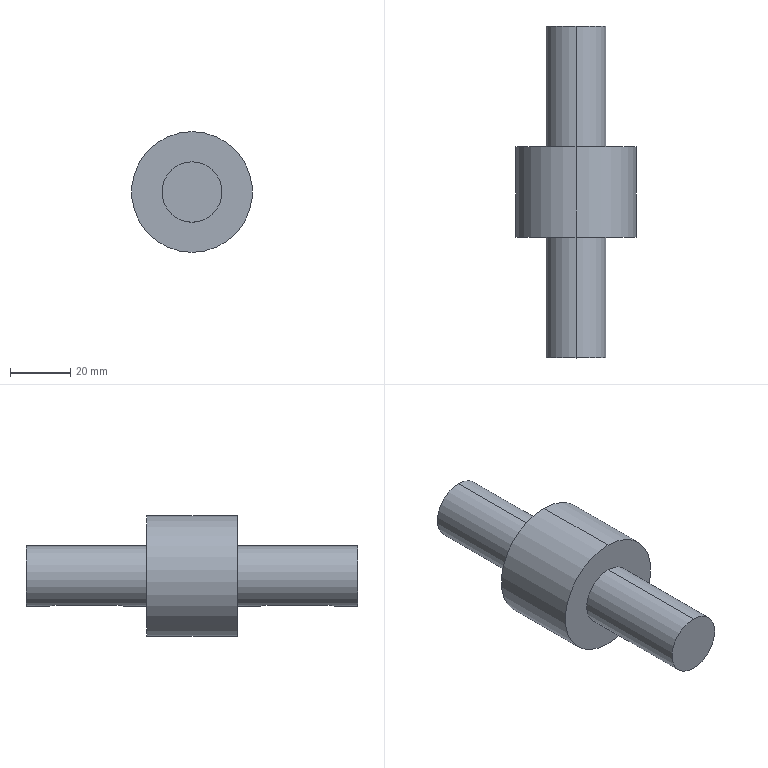Part | SolidWorks | features ICE 1, MirrorPattern 1, Revolution 1 | 1 solid | 20 faces | box 40 x 110 x 40 mm | volume 62258 mm3 | cylinder 10 | plane 10 | commonest cylinder face diameters 5 x4 20 x4 40 x2
STEP:
#1=CARTESIAN_POINT('',(0.,-15.,20.));
#2=VERTEX_POINT('',#1);
#3=CARTESIAN_POINT('',(0.,-15.,-20.));
#4=VERTEX_POINT('',#3);
#5=CARTESIAN_POINT('',(0.,-15.,0.));
#6=DIRECTION('',(0.,1.,0.));
#7=DIRECTION('',(0.,0.,1.));
#8=AXIS2_PLACEMENT_3D('',#5,#6,#7);
#9=CIRCLE('',#8,20.);
#10=EDGE_CURVE('',#2,#4,#9,.T.);
#11=ORIENTED_EDGE('',*,*,#10,.T.);
#12=CARTESIAN_POINT('',(0.,15.,-20.));
#13=VERTEX_POINT('',#12);
#14=CARTESIAN_POINT('',(0.,189.93,-20.));
#15=DIRECTION('',(0.,1.,0.));
#16=VECTOR('',#15,1000.);
#17=LINE('',#14,#16);
#18=EDGE_CURVE('',#4,#13,#17,.T.);
#19=ORIENTED_EDGE('',*,*,#18,.T.);
#20=CARTESIAN_POINT('',(0.,15.,20.));
#21=VERTEX_POINT('',#20);
#22=CARTESIAN_POINT('',(0.,15.,0.));
#23=DIRECTION('',(0.,1.,0.));
#24=DIRECTION('',(0.,0.,1.));
#25=AXIS2_PLACEMENT_3D('',#22,#23,#24);
#26=CIRCLE('',#25,20.);
#27=EDGE_CURVE('',#21,#13,#26,.T.);
#28=ORIENTED_EDGE('',*,*,#27,.F.);
#29=CARTESIAN_POINT('',(0.,189.93,20.));
#30=DIRECTION('',(0.,1.,0.));
#31=VECTOR('',#30,1000.);
#32=LINE('',#29,#31);
#33=EDGE_CURVE('',#2,#21,#32,.T.);
#34=ORIENTED_EDGE('',*,*,#33,.F.);
#35=EDGE_LOOP('',(#11,#19,#28,#34));
#36=FACE_OUTER_BOUND('',#35,.T.);
#37=CARTESIAN_POINT('',(0.,189.93,0.));
#38=DIRECTION('',(0.,1.,0.));
#39=DIRECTION('',(0.,0.,1.));
#40=AXIS2_PLACEMENT_3D('',#37,#38,#39);
#41=CYLINDRICAL_SURFACE('',#40,20.);
#42=ADVANCED_FACE('',(#36),#41,.T.);
#43=CARTESIAN_POINT('',(0.,15.,10.));
#44=VERTEX_POINT('',#43);
#45=CARTESIAN_POINT('',(0.,15.,-10.));
#46=VERTEX_POINT('',#45);
#47=CARTESIAN_POINT('',(0.,15.,0.));
#48=DIRECTION('',(0.,1.,0.));
#49=DIRECTION('',(0.,0.,1.));
#50=AXIS2_PLACEMENT_3D('',#47,#48,#49);
#51=CIRCLE('',#50,10.);
#52=EDGE_CURVE('',#44,#46,#51,.T.);
#53=ORIENTED_EDGE('',*,*,#52,.T.);
#54=CARTESIAN_POINT('',(0.,22.5,-10.));
#55=VERTEX_POINT('',#54);
#56=CARTESIAN_POINT('',(0.,189.93,-10.));
#57=DIRECTION('',(0.,1.,0.));
#58=VECTOR('',#57,1000.);
#59=LINE('',#56,#58);
#60=EDGE_CURVE('',#46,#55,#59,.T.);
#61=ORIENTED_EDGE('',*,*,#60,.T.);
#62=CARTESIAN_POINT('',(2.5,25.,-9.682));
#63=VERTEX_POINT('',#62);
#64=CARTESIAN_POINT('',(2.5,25.,-9.682));
#65=CARTESIAN_POINT('',(2.5,24.834,-9.682));
#66=CARTESIAN_POINT('',(2.484,24.671,-9.687));
#67=CARTESIAN_POINT('',(2.42,24.351,-9.703));
#68=CARTESIAN_POINT('',(2.371,24.191,-9.715));
#69=CARTESIAN_POINT('',(2.245,23.889,-9.745));
#70=CARTESIAN_POINT('',(2.169,23.745,-9.762));
#71=CARTESIAN_POINT('',(1.987,23.474,-9.801));
#72=CARTESIAN_POINT('',(1.882,23.346,-9.822));
#73=CARTESIAN_POINT('',(1.537,23.002,-9.884));
#74=CARTESIAN_POINT('',(1.259,22.816,-9.925));
#75=CARTESIAN_POINT('',(0.8081,22.629,-9.968));
#76=CARTESIAN_POINT('',(0.6497,22.58,-9.98));
#77=CARTESIAN_POINT('',(0.3266,22.516,-9.996));
#78=CARTESIAN_POINT('',(0.1638,22.5,-10.));
#79=CARTESIAN_POINT('',(0.,22.5,-10.));
#80=B_SPLINE_CURVE_WITH_KNOTS('',3,(#64,#65,#66,#67,#68,#69,#70,#71,#72,#73,#74,#75,#76,#77,#78,#79),.UNSPECIFIED.,.F.,.F.,(4,2,2,2,2,2,2,4),(0.,0.0004906,0.0009812,0.001472,0.001962,0.002944,0.003434,0.003925),.UNSPECIFIED.);
#81=EDGE_CURVE('',#63,#55,#80,.T.);
#82=ORIENTED_EDGE('',*,*,#81,.F.);
#83=CARTESIAN_POINT('',(2.5,45.,-9.682));
#84=VERTEX_POINT('',#83);
#85=CARTESIAN_POINT('',(2.5,189.93,-9.682));
#86=DIRECTION('',(0.,-1.,0.));
#87=VECTOR('',#86,1000.);
#88=LINE('',#85,#87);
#89=EDGE_CURVE('',#84,#63,#88,.T.);
#90=ORIENTED_EDGE('',*,*,#89,.F.);
#91=CARTESIAN_POINT('',(0.,47.5,-10.));
#92=VERTEX_POINT('',#91);
#93=CARTESIAN_POINT('',(0.,47.5,-10.));
#94=CARTESIAN_POINT('',(0.1637,47.5,-10.));
#95=CARTESIAN_POINT('',(0.3299,47.484,-9.996));
#96=CARTESIAN_POINT('',(0.6508,47.419,-9.98));
#97=CARTESIAN_POINT('',(0.8069,47.372,-9.969));
#98=CARTESIAN_POINT('',(1.262,47.183,-9.925));
#99=CARTESIAN_POINT('',(1.536,46.999,-9.884));
#100=CARTESIAN_POINT('',(1.884,46.652,-9.822));
#101=CARTESIAN_POINT('',(1.986,46.527,-9.801));
#102=CARTESIAN_POINT('',(2.167,46.257,-9.763));
#103=CARTESIAN_POINT('',(2.246,46.11,-9.745));
#104=CARTESIAN_POINT('',(2.371,45.809,-9.715));
#105=CARTESIAN_POINT('',(2.419,45.653,-9.703));
#106=CARTESIAN_POINT('',(2.483,45.332,-9.687));
#107=CARTESIAN_POINT('',(2.5,45.166,-9.682));
#108=CARTESIAN_POINT('',(2.5,45.,-9.682));
#109=B_SPLINE_CURVE_WITH_KNOTS('',3,(#93,#94,#95,#96,#97,#98,#99,#100,#101,#102,#103,#104,#105,#106,#107,#108),.UNSPECIFIED.,.F.,.F.,(4,2,2,2,2,2,2,4),(0.003925,0.004415,0.004905,0.005885,0.006375,0.006865,0.007355,0.007845),.UNSPECIFIED.);
#110=EDGE_CURVE('',#92,#84,#109,.T.);
#111=ORIENTED_EDGE('',*,*,#110,.F.);
#112=CARTESIAN_POINT('',(0.,55.,-10.));
#113=VERTEX_POINT('',#112);
#114=CARTESIAN_POINT('',(0.,189.93,-10.));
#115=DIRECTION('',(0.,1.,0.));
#116=VECTOR('',#115,1000.);
#117=LINE('',#114,#116);
#118=EDGE_CURVE('',#92,#113,#117,.T.);
#119=ORIENTED_EDGE('',*,*,#118,.T.);
#120=CARTESIAN_POINT('',(0.,55.,10.));
#121=VERTEX_POINT('',#120);
#122=CARTESIAN_POINT('',(0.,55.,0.));
#123=DIRECTION('',(0.,1.,0.));
#124=DIRECTION('',(0.,0.,1.));
#125=AXIS2_PLACEMENT_3D('',#122,#123,#124);
#126=CIRCLE('',#125,10.);
#127=EDGE_CURVE('',#121,#113,#126,.T.);
#128=ORIENTED_EDGE('',*,*,#127,.F.);
#129=CARTESIAN_POINT('',(0.,189.93,10.));
#130=DIRECTION('',(0.,1.,0.));
#131=VECTOR('',#130,1000.);
#132=LINE('',#129,#131);
#133=EDGE_CURVE('',#44,#121,#132,.T.);
#134=ORIENTED_EDGE('',*,*,#133,.F.);
#135=EDGE_LOOP('',(#53,#61,#82,#90,#111,#119,#128,#134));
#136=FACE_OUTER_BOUND('',#135,.T.);
#137=CARTESIAN_POINT('',(0.,189.93,0.));
#138=DIRECTION('',(0.,1.,0.));
#139=DIRECTION('',(0.,0.,1.));
#140=AXIS2_PLACEMENT_3D('',#137,#138,#139);
#141=CYLINDRICAL_SURFACE('',#140,10.);
#142=ADVANCED_FACE('',(#136),#141,.T.);
#143=CARTESIAN_POINT('',(0.,-55.,10.));
#144=VERTEX_POINT('',#143);
#145=CARTESIAN_POINT('',(0.,-55.,-10.));
#146=VERTEX_POINT('',#145);
#147=CARTESIAN_POINT('',(0.,-55.,0.));
#148=DIRECTION('',(0.,1.,0.));
#149=DIRECTION('',(0.,0.,1.));
#150=AXIS2_PLACEMENT_3D('',#147,#148,#149);
#151=CIRCLE('',#150,10.);
#152=EDGE_CURVE('',#144,#146,#151,.T.);
#153=ORIENTED_EDGE('',*,*,#152,.T.);
#154=CARTESIAN_POINT('',(0.,-47.5,-10.));
#155=VERTEX_POINT('',#154);
#156=CARTESIAN_POINT('',(0.,189.93,-10.));
#157=DIRECTION('',(0.,1.,0.));
#158=VECTOR('',#157,1000.);
#159=LINE('',#156,#158);
#160=EDGE_CURVE('',#146,#155,#159,.T.);
#161=ORIENTED_EDGE('',*,*,#160,.T.);
#162=CARTESIAN_POINT('',(2.5,-45.,-9.682));
#163=VERTEX_POINT('',#162);
#164=CARTESIAN_POINT('',(0.,-47.5,-10.));
#165=CARTESIAN_POINT('',(0.1637,-47.5,-10.));
#166=CARTESIAN_POINT('',(0.3299,-47.484,-9.996));
#167=CARTESIAN_POINT('',(0.6508,-47.419,-9.98));
#168=CARTESIAN_POINT('',(0.8069,-47.372,-9.969));
#169=CARTESIAN_POINT('',(1.262,-47.183,-9.925));
#170=CARTESIAN_POINT('',(1.536,-46.999,-9.884));
#171=CARTESIAN_POINT('',(1.884,-46.652,-9.822));
#172=CARTESIAN_POINT('',(1.986,-46.527,-9.801));
#173=CARTESIAN_POINT('',(2.167,-46.257,-9.763));
#174=CARTESIAN_POINT('',(2.246,-46.11,-9.745));
#175=CARTESIAN_POINT('',(2.371,-45.809,-9.715));
#176=CARTESIAN_POINT('',(2.419,-45.653,-9.703));
#177=CARTESIAN_POINT('',(2.483,-45.332,-9.687));
#178=CARTESIAN_POINT('',(2.5,-45.166,-9.682));
#179=CARTESIAN_POINT('',(2.5,-45.,-9.682));
#180=B_SPLINE_CURVE_WITH_KNOTS('',3,(#164,#165,#166,#167,#168,#169,#170,#171,#172,#173,#174,#175,#176,#177,#178,#179),.UNSPECIFIED.,.F.,.F.,(4,2,2,2,2,2,2,4),(0.003925,0.004415,0.004905,0.005885,0.006375,0.006865,0.007355,0.007845),.UNSPECIFIED.);
#181=EDGE_CURVE('',#155,#163,#180,.T.);
#182=ORIENTED_EDGE('',*,*,#181,.T.);
#183=CARTESIAN_POINT('',(2.5,-25.,-9.682));
#184=VERTEX_POINT('',#183);
#185=CARTESIAN_POINT('',(2.5,189.93,-9.682));
#186=DIRECTION('',(0.,1.,0.));
#187=VECTOR('',#186,1000.);
#188=LINE('',#185,#187);
#189=EDGE_CURVE('',#163,#184,#188,.T.);
#190=ORIENTED_EDGE('',*,*,#189,.T.);
#191=CARTESIAN_POINT('',(0.,-22.5,-10.));
#192=VERTEX_POINT('',#191);
#193=CARTESIAN_POINT('',(2.5,-25.,-9.682));
#194=CARTESIAN_POINT('',(2.5,-24.834,-9.682));
#195=CARTESIAN_POINT('',(2.484,-24.671,-9.687));
#196=CARTESIAN_POINT('',(2.42,-24.351,-9.703));
#197=CARTESIAN_POINT('',(2.371,-24.191,-9.715));
#198=CARTESIAN_POINT('',(2.245,-23.889,-9.745));
#199=CARTESIAN_POINT('',(2.169,-23.745,-9.762));
#200=CARTESIAN_POINT('',(1.987,-23.474,-9.801));
#201=CARTESIAN_POINT('',(1.882,-23.346,-9.822));
#202=CARTESIAN_POINT('',(1.537,-23.002,-9.884));
#203=CARTESIAN_POINT('',(1.259,-22.816,-9.925));
#204=CARTESIAN_POINT('',(0.8081,-22.629,-9.968));
#205=CARTESIAN_POINT('',(0.6497,-22.58,-9.98));
#206=CARTESIAN_POINT('',(0.3266,-22.516,-9.996));
#207=CARTESIAN_POINT('',(0.1638,-22.5,-10.));
#208=CARTESIAN_POINT('',(0.,-22.5,-10.));
#209=B_SPLINE_CURVE_WITH_KNOTS('',3,(#193,#194,#195,#196,#197,#198,#199,#200,#201,#202,#203,#204,#205,#206,#207,#208),.UNSPECIFIED.,.F.,.F.,(4,2,2,2,2,2,2,4),(0.,0.0004906,0.0009812,0.001472,0.001962,0.002944,0.003434,0.003925),.UNSPECIFIED.);
#210=EDGE_CURVE('',#184,#192,#209,.T.);
#211=ORIENTED_EDGE('',*,*,#210,.T.);
#212=CARTESIAN_POINT('',(0.,-15.,-10.));
#213=VERTEX_POINT('',#212);
#214=CARTESIAN_POINT('',(0.,189.93,-10.));
#215=DIRECTION('',(0.,1.,0.));
#216=VECTOR('',#215,1000.);
#217=LINE('',#214,#216);
#218=EDGE_CURVE('',#192,#213,#217,.T.);
#219=ORIENTED_EDGE('',*,*,#218,.T.);
#220=CARTESIAN_POINT('',(0.,-15.,10.));
#221=VERTEX_POINT('',#220);
#222=CARTESIAN_POINT('',(0.,-15.,0.));
#223=DIRECTION('',(0.,1.,0.));
#224=DIRECTION('',(0.,0.,1.));
#225=AXIS2_PLACEMENT_3D('',#222,#223,#224);
#226=CIRCLE('',#225,10.);
#227=EDGE_CURVE('',#221,#213,#226,.T.);
#228=ORIENTED_EDGE('',*,*,#227,.F.);
#229=CARTESIAN_POINT('',(0.,189.93,10.));
#230=DIRECTION('',(0.,1.,0.));
#231=VECTOR('',#230,1000.);
#232=LINE('',#229,#231);
#233=EDGE_CURVE('',#144,#221,#232,.T.);
#234=ORIENTED_EDGE('',*,*,#233,.F.);
#235=EDGE_LOOP('',(#153,#161,#182,#190,#211,#219,#228,#234));
#236=FACE_OUTER_BOUND('',#235,.T.);
#237=CARTESIAN_POINT('',(0.,189.93,0.));
#238=DIRECTION('',(0.,1.,0.));
#239=DIRECTION('',(0.,0.,1.));
#240=AXIS2_PLACEMENT_3D('',#237,#238,#239);
#241=CYLINDRICAL_SURFACE('',#240,10.);
#242=ADVANCED_FACE('',(#236),#241,.T.);
#243=ORIENTED_EDGE('',*,*,#160,.F.);
#244=CARTESIAN_POINT('',(0.,-55.,0.));
#245=DIRECTION('',(0.,1.,0.));
#246=DIRECTION('',(0.,0.,1.));
#247=AXIS2_PLACEMENT_3D('',#244,#245,#246);
#248=CIRCLE('',#247,10.);
#249=EDGE_CURVE('',#146,#144,#248,.T.);
#250=ORIENTED_EDGE('',*,*,#249,.T.);
#251=ORIENTED_EDGE('',*,*,#233,.T.);
#252=CARTESIAN_POINT('',(0.,-15.,0.));
#253=DIRECTION('',(0.,1.,0.));
#254=DIRECTION('',(0.,0.,1.));
#255=AXIS2_PLACEMENT_3D('',#252,#253,#254);
#256=CIRCLE('',#255,10.);
#257=EDGE_CURVE('',#213,#221,#256,.T.);
#258=ORIENTED_EDGE('',*,*,#257,.F.);
#259=ORIENTED_EDGE('',*,*,#218,.F.);
#260=CARTESIAN_POINT('',(-2.5,-25.,-9.682));
#261=VERTEX_POINT('',#260);
#262=CARTESIAN_POINT('',(0.,-22.5,-10.));
#263=CARTESIAN_POINT('',(-0.1637,-22.5,-10.));
#264=CARTESIAN_POINT('',(-0.3299,-22.516,-9.996));
#265=CARTESIAN_POINT('',(-0.6508,-22.581,-9.98));
#266=CARTESIAN_POINT('',(-0.8069,-22.628,-9.969));
#267=CARTESIAN_POINT('',(-1.262,-22.817,-9.925));
#268=CARTESIAN_POINT('',(-1.536,-23.001,-9.884));
#269=CARTESIAN_POINT('',(-1.884,-23.348,-9.822));
#270=CARTESIAN_POINT('',(-1.986,-23.473,-9.801));
#271=CARTESIAN_POINT('',(-2.167,-23.743,-9.763));
#272=CARTESIAN_POINT('',(-2.246,-23.89,-9.745));
#273=CARTESIAN_POINT('',(-2.371,-24.191,-9.715));
#274=CARTESIAN_POINT('',(-2.419,-24.347,-9.703));
#275=CARTESIAN_POINT('',(-2.483,-24.668,-9.687));
#276=CARTESIAN_POINT('',(-2.5,-24.834,-9.682));
#277=CARTESIAN_POINT('',(-2.5,-25.,-9.682));
#278=B_SPLINE_CURVE_WITH_KNOTS('',3,(#262,#263,#264,#265,#266,#267,#268,#269,#270,#271,#272,#273,#274,#275,#276,#277),.UNSPECIFIED.,.F.,.F.,(4,2,2,2,2,2,2,4),(0.003925,0.004415,0.004905,0.005885,0.006375,0.006865,0.007355,0.007845),.UNSPECIFIED.);
#279=EDGE_CURVE('',#192,#261,#278,.T.);
#280=ORIENTED_EDGE('',*,*,#279,.T.);
#281=CARTESIAN_POINT('',(-2.5,-45.,-9.682));
#282=VERTEX_POINT('',#281);
#283=CARTESIAN_POINT('',(-2.5,189.93,-9.682));
#284=DIRECTION('',(0.,-1.,0.));
#285=VECTOR('',#284,1000.);
#286=LINE('',#283,#285);
#287=EDGE_CURVE('',#261,#282,#286,.T.);
#288=ORIENTED_EDGE('',*,*,#287,.T.);
#289=CARTESIAN_POINT('',(-2.5,-45.,-9.682));
#290=CARTESIAN_POINT('',(-2.5,-45.166,-9.682));
#291=CARTESIAN_POINT('',(-2.484,-45.329,-9.687));
#292=CARTESIAN_POINT('',(-2.42,-45.649,-9.703));
#293=CARTESIAN_POINT('',(-2.371,-45.809,-9.715));
#294=CARTESIAN_POINT('',(-2.245,-46.111,-9.745));
#295=CARTESIAN_POINT('',(-2.169,-46.255,-9.762));
#296=CARTESIAN_POINT('',(-1.987,-46.526,-9.801));
#297=CARTESIAN_POINT('',(-1.882,-46.654,-9.822));
#298=CARTESIAN_POINT('',(-1.537,-46.998,-9.884));
#299=CARTESIAN_POINT('',(-1.259,-47.184,-9.925));
#300=CARTESIAN_POINT('',(-0.8081,-47.371,-9.968));
#301=CARTESIAN_POINT('',(-0.6497,-47.42,-9.98));
#302=CARTESIAN_POINT('',(-0.3266,-47.484,-9.996));
#303=CARTESIAN_POINT('',(-0.1638,-47.5,-10.));
#304=CARTESIAN_POINT('',(0.,-47.5,-10.));
#305=B_SPLINE_CURVE_WITH_KNOTS('',3,(#289,#290,#291,#292,#293,#294,#295,#296,#297,#298,#299,#300,#301,#302,#303,#304),.UNSPECIFIED.,.F.,.F.,(4,2,2,2,2,2,2,4),(0.,0.0004906,0.0009812,0.001472,0.001962,0.002944,0.003434,0.003925),.UNSPECIFIED.);
#306=EDGE_CURVE('',#282,#155,#305,.T.);
#307=ORIENTED_EDGE('',*,*,#306,.T.);
#308=EDGE_LOOP('',(#243,#250,#251,#258,#259,#280,#288,#307));
#309=FACE_OUTER_BOUND('',#308,.T.);
#310=CARTESIAN_POINT('',(0.,189.93,0.));
#311=DIRECTION('',(0.,1.,0.));
#312=DIRECTION('',(0.,0.,1.));
#313=AXIS2_PLACEMENT_3D('',#310,#311,#312);
#314=CYLINDRICAL_SURFACE('',#313,10.);
#315=ADVANCED_FACE('',(#309),#314,.T.);
#316=ORIENTED_EDGE('',*,*,#127,.T.);
#317=CARTESIAN_POINT('',(0.,55.,0.));
#318=DIRECTION('',(0.,1.,0.));
#319=DIRECTION('',(0.,0.,1.));
#320=AXIS2_PLACEMENT_3D('',#317,#318,#319);
#321=CIRCLE('',#320,10.);
#322=EDGE_CURVE('',#113,#121,#321,.T.);
#323=ORIENTED_EDGE('',*,*,#322,.T.);
#324=EDGE_LOOP('',(#316,#323));
#325=FACE_OUTER_BOUND('',#324,.T.);
#326=CARTESIAN_POINT('',(0.,55.,0.));
#327=DIRECTION('',(0.,1.,0.));
#328=DIRECTION('',(0.,0.,1.));
#329=AXIS2_PLACEMENT_3D('',#326,#327,#328);
#330=PLANE('',#329);
#331=ADVANCED_FACE('',(#325),#330,.T.);
#332=ORIENTED_EDGE('',*,*,#60,.F.);
#333=CARTESIAN_POINT('',(0.,15.,0.));
#334=DIRECTION('',(0.,1.,0.));
#335=DIRECTION('',(0.,0.,1.));
#336=AXIS2_PLACEMENT_3D('',#333,#334,#335);
#337=CIRCLE('',#336,10.);
#338=EDGE_CURVE('',#46,#44,#337,.T.);
#339=ORIENTED_EDGE('',*,*,#338,.T.);
#340=ORIENTED_EDGE('',*,*,#133,.T.);
#341=ORIENTED_EDGE('',*,*,#322,.F.);
#342=ORIENTED_EDGE('',*,*,#118,.F.);
#343=CARTESIAN_POINT('',(-2.5,45.,-9.682));
#344=VERTEX_POINT('',#343);
#345=CARTESIAN_POINT('',(-2.5,45.,-9.682));
#346=CARTESIAN_POINT('',(-2.5,45.166,-9.682));
#347=CARTESIAN_POINT('',(-2.484,45.329,-9.687));
#348=CARTESIAN_POINT('',(-2.42,45.649,-9.703));
#349=CARTESIAN_POINT('',(-2.371,45.809,-9.715));
#350=CARTESIAN_POINT('',(-2.245,46.111,-9.745));
#351=CARTESIAN_POINT('',(-2.169,46.255,-9.762));
#352=CARTESIAN_POINT('',(-1.987,46.526,-9.801));
#353=CARTESIAN_POINT('',(-1.882,46.654,-9.822));
#354=CARTESIAN_POINT('',(-1.537,46.998,-9.884));
#355=CARTESIAN_POINT('',(-1.259,47.184,-9.925));
#356=CARTESIAN_POINT('',(-0.8081,47.371,-9.968));
#357=CARTESIAN_POINT('',(-0.6497,47.42,-9.98));
#358=CARTESIAN_POINT('',(-0.3266,47.484,-9.996));
#359=CARTESIAN_POINT('',(-0.1638,47.5,-10.));
#360=CARTESIAN_POINT('',(0.,47.5,-10.));
#361=B_SPLINE_CURVE_WITH_KNOTS('',3,(#345,#346,#347,#348,#349,#350,#351,#352,#353,#354,#355,#356,#357,#358,#359,#360),.UNSPECIFIED.,.F.,.F.,(4,2,2,2,2,2,2,4),(0.,0.0004906,0.0009812,0.001472,0.001962,0.002944,0.003434,0.003925),.UNSPECIFIED.);
#362=EDGE_CURVE('',#344,#92,#361,.T.);
#363=ORIENTED_EDGE('',*,*,#362,.F.);
#364=CARTESIAN_POINT('',(-2.5,25.,-9.682));
#365=VERTEX_POINT('',#364);
#366=CARTESIAN_POINT('',(-2.5,189.93,-9.682));
#367=DIRECTION('',(0.,1.,0.));
#368=VECTOR('',#367,1000.);
#369=LINE('',#366,#368);
#370=EDGE_CURVE('',#365,#344,#369,.T.);
#371=ORIENTED_EDGE('',*,*,#370,.F.);
#372=CARTESIAN_POINT('',(0.,22.5,-10.));
#373=CARTESIAN_POINT('',(-0.1637,22.5,-10.));
#374=CARTESIAN_POINT('',(-0.3299,22.516,-9.996));
#375=CARTESIAN_POINT('',(-0.6508,22.581,-9.98));
#376=CARTESIAN_POINT('',(-0.8069,22.628,-9.969));
#377=CARTESIAN_POINT('',(-1.262,22.817,-9.925));
#378=CARTESIAN_POINT('',(-1.536,23.001,-9.884));
#379=CARTESIAN_POINT('',(-1.884,23.348,-9.822));
#380=CARTESIAN_POINT('',(-1.986,23.473,-9.801));
#381=CARTESIAN_POINT('',(-2.167,23.743,-9.763));
#382=CARTESIAN_POINT('',(-2.246,23.89,-9.745));
#383=CARTESIAN_POINT('',(-2.371,24.191,-9.715));
#384=CARTESIAN_POINT('',(-2.419,24.347,-9.703));
#385=CARTESIAN_POINT('',(-2.483,24.668,-9.687));
#386=CARTESIAN_POINT('',(-2.5,24.834,-9.682));
#387=CARTESIAN_POINT('',(-2.5,25.,-9.682));
#388=B_SPLINE_CURVE_WITH_KNOTS('',3,(#372,#373,#374,#375,#376,#377,#378,#379,#380,#381,#382,#383,#384,#385,#386,#387),.UNSPECIFIED.,.F.,.F.,(4,2,2,2,2,2,2,4),(0.003925,0.004415,0.004905,0.005885,0.006375,0.006865,0.007355,0.007845),.UNSPECIFIED.);
#389=EDGE_CURVE('',#55,#365,#388,.T.);
#390=ORIENTED_EDGE('',*,*,#389,.F.);
#391=EDGE_LOOP('',(#332,#339,#340,#341,#342,#363,#371,#390));
#392=FACE_OUTER_BOUND('',#391,.T.);
#393=CARTESIAN_POINT('',(0.,189.93,0.));
#394=DIRECTION('',(0.,1.,0.));
#395=DIRECTION('',(0.,0.,1.));
#396=AXIS2_PLACEMENT_3D('',#393,#394,#395);
#397=CYLINDRICAL_SURFACE('',#396,10.);
#398=ADVANCED_FACE('',(#392),#397,.T.);
#399=ORIENTED_EDGE('',*,*,#27,.T.);
#400=CARTESIAN_POINT('',(0.,15.,0.));
#401=DIRECTION('',(0.,1.,0.));
#402=DIRECTION('',(0.,0.,1.));
#403=AXIS2_PLACEMENT_3D('',#400,#401,#402);
#404=CIRCLE('',#403,20.);
#405=EDGE_CURVE('',#13,#21,#404,.T.);
#406=ORIENTED_EDGE('',*,*,#405,.T.);
#407=EDGE_LOOP('',(#399,#406));
#408=FACE_OUTER_BOUND('',#407,.T.);
#409=ORIENTED_EDGE('',*,*,#52,.F.);
#410=ORIENTED_EDGE('',*,*,#338,.F.);
#411=EDGE_LOOP('',(#409,#410));
#412=FACE_BOUND('',#411,.T.);
#413=CARTESIAN_POINT('',(0.,15.,10.));
#414=DIRECTION('',(0.,1.,0.));
#415=DIRECTION('',(0.,0.,1.));
#416=AXIS2_PLACEMENT_3D('',#413,#414,#415);
#417=PLANE('',#416);
#418=ADVANCED_FACE('',(#408,#412),#417,.T.);
#419=ORIENTED_EDGE('',*,*,#18,.F.);
#420=CARTESIAN_POINT('',(0.,-15.,0.));
#421=DIRECTION('',(0.,1.,0.));
#422=DIRECTION('',(0.,0.,1.));
#423=AXIS2_PLACEMENT_3D('',#420,#421,#422);
#424=CIRCLE('',#423,20.);
#425=EDGE_CURVE('',#4,#2,#424,.T.);
#426=ORIENTED_EDGE('',*,*,#425,.T.);
#427=ORIENTED_EDGE('',*,*,#33,.T.);
#428=ORIENTED_EDGE('',*,*,#405,.F.);
#429=EDGE_LOOP('',(#419,#426,#427,#428));
#430=FACE_OUTER_BOUND('',#429,.T.);
#431=CARTESIAN_POINT('',(0.,189.93,0.));
#432=DIRECTION('',(0.,1.,0.));
#433=DIRECTION('',(0.,0.,1.));
#434=AXIS2_PLACEMENT_3D('',#431,#432,#433);
#435=CYLINDRICAL_SURFACE('',#434,20.);
#436=ADVANCED_FACE('',(#430),#435,.T.);
#437=ORIENTED_EDGE('',*,*,#227,.T.);
#438=ORIENTED_EDGE('',*,*,#257,.T.);
#439=EDGE_LOOP('',(#437,#438));
#440=FACE_BOUND('',#439,.T.);
#441=ORIENTED_EDGE('',*,*,#10,.F.);
#442=ORIENTED_EDGE('',*,*,#425,.F.);
#443=EDGE_LOOP('',(#441,#442));
#444=FACE_OUTER_BOUND('',#443,.T.);
#445=CARTESIAN_POINT('',(0.,-15.,20.));
#446=DIRECTION('',(0.,-1.,0.));
#447=DIRECTION('',(0.,0.,-1.));
#448=AXIS2_PLACEMENT_3D('',#445,#446,#447);
#449=PLANE('',#448);
#450=ADVANCED_FACE('',(#440,#444),#449,.T.);
#451=ORIENTED_EDGE('',*,*,#152,.F.);
#452=ORIENTED_EDGE('',*,*,#249,.F.);
#453=EDGE_LOOP('',(#451,#452));
#454=FACE_OUTER_BOUND('',#453,.T.);
#455=CARTESIAN_POINT('',(0.,-55.,10.));
#456=DIRECTION('',(0.,-1.,0.));
#457=DIRECTION('',(0.,0.,-1.));
#458=AXIS2_PLACEMENT_3D('',#455,#456,#457);
#459=PLANE('',#458);
#460=ADVANCED_FACE('',(#454),#459,.T.);
#461=CARTESIAN_POINT('',(-2.5,45.,-7.5));
#462=VERTEX_POINT('',#461);
#463=CARTESIAN_POINT('',(-2.5,45.,-7.5));
#464=DIRECTION('',(0.,0.,-1.));
#465=VECTOR('',#464,1000.);
#466=LINE('',#463,#465);
#467=EDGE_CURVE('',#462,#344,#466,.T.);
#468=ORIENTED_EDGE('',*,*,#467,.T.);
#469=ORIENTED_EDGE('',*,*,#362,.T.);
#470=ORIENTED_EDGE('',*,*,#110,.T.);
#471=CARTESIAN_POINT('',(2.5,45.,-7.5));
#472=VERTEX_POINT('',#471);
#473=CARTESIAN_POINT('',(2.5,45.,-7.5));
#474=DIRECTION('',(0.,0.,-1.));
#475=VECTOR('',#474,1000.);
#476=LINE('',#473,#475);
#477=EDGE_CURVE('',#472,#84,#476,.T.);
#478=ORIENTED_EDGE('',*,*,#477,.F.);
#479=CARTESIAN_POINT('',(0.,45.,-7.5));
#480=DIRECTION('',(0.,0.,-1.));
#481=DIRECTION('',(-1.,0.,0.));
#482=AXIS2_PLACEMENT_3D('',#479,#480,#481);
#483=CIRCLE('',#482,2.5);
#484=EDGE_CURVE('',#462,#472,#483,.T.);
#485=ORIENTED_EDGE('',*,*,#484,.F.);
#486=EDGE_LOOP('',(#468,#469,#470,#478,#485));
#487=FACE_OUTER_BOUND('',#486,.T.);
#488=CARTESIAN_POINT('',(0.,45.,-7.5));
#489=DIRECTION('',(0.,0.,-1.));
#490=DIRECTION('',(-1.,0.,0.));
#491=AXIS2_PLACEMENT_3D('',#488,#489,#490);
#492=CYLINDRICAL_SURFACE('',#491,2.5);
#493=ADVANCED_FACE('',(#487),#492,.F.);
#494=ORIENTED_EDGE('',*,*,#370,.T.);
#495=ORIENTED_EDGE('',*,*,#467,.F.);
#496=CARTESIAN_POINT('',(-2.5,25.,-7.5));
#497=VERTEX_POINT('',#496);
#498=CARTESIAN_POINT('',(-2.5,45.,-7.5));
#499=DIRECTION('',(0.,1.,0.));
#500=VECTOR('',#499,1000.);
#501=LINE('',#498,#500);
#502=EDGE_CURVE('',#497,#462,#501,.T.);
#503=ORIENTED_EDGE('',*,*,#502,.F.);
#504=CARTESIAN_POINT('',(-2.5,25.,-7.5));
#505=DIRECTION('',(0.,0.,-1.));
#506=VECTOR('',#505,1000.);
#507=LINE('',#504,#506);
#508=EDGE_CURVE('',#497,#365,#507,.T.);
#509=ORIENTED_EDGE('',*,*,#508,.T.);
#510=EDGE_LOOP('',(#494,#495,#503,#509));
#511=FACE_OUTER_BOUND('',#510,.T.);
#512=CARTESIAN_POINT('',(-2.5,45.,-7.5));
#513=DIRECTION('',(-1.,0.,0.));
#514=DIRECTION('',(0.,-1.,0.));
#515=AXIS2_PLACEMENT_3D('',#512,#513,#514);
#516=PLANE('',#515);
#517=ADVANCED_FACE('',(#511),#516,.F.);
#518=CARTESIAN_POINT('',(2.5,25.,-7.5));
#519=VERTEX_POINT('',#518);
#520=CARTESIAN_POINT('',(2.5,25.,-7.5));
#521=DIRECTION('',(0.,0.,-1.));
#522=VECTOR('',#521,1000.);
#523=LINE('',#520,#522);
#524=EDGE_CURVE('',#519,#63,#523,.T.);
#525=ORIENTED_EDGE('',*,*,#524,.T.);
#526=ORIENTED_EDGE('',*,*,#81,.T.);
#527=ORIENTED_EDGE('',*,*,#389,.T.);
#528=ORIENTED_EDGE('',*,*,#508,.F.);
#529=CARTESIAN_POINT('',(0.,25.,-7.5));
#530=DIRECTION('',(0.,0.,-1.));
#531=DIRECTION('',(-1.,0.,0.));
#532=AXIS2_PLACEMENT_3D('',#529,#530,#531);
#533=CIRCLE('',#532,2.5);
#534=EDGE_CURVE('',#519,#497,#533,.T.);
#535=ORIENTED_EDGE('',*,*,#534,.F.);
#536=EDGE_LOOP('',(#525,#526,#527,#528,#535));
#537=FACE_OUTER_BOUND('',#536,.T.);
#538=CARTESIAN_POINT('',(0.,25.,-7.5));
#539=DIRECTION('',(0.,0.,-1.));
#540=DIRECTION('',(-1.,0.,0.));
#541=AXIS2_PLACEMENT_3D('',#538,#539,#540);
#542=CYLINDRICAL_SURFACE('',#541,2.5);
#543=ADVANCED_FACE('',(#537),#542,.F.);
#544=ORIENTED_EDGE('',*,*,#89,.T.);
#545=ORIENTED_EDGE('',*,*,#524,.F.);
#546=CARTESIAN_POINT('',(2.5,45.,-7.5));
#547=DIRECTION('',(0.,-1.,0.));
#548=VECTOR('',#547,1000.);
#549=LINE('',#546,#548);
#550=EDGE_CURVE('',#472,#519,#549,.T.);
#551=ORIENTED_EDGE('',*,*,#550,.F.);
#552=ORIENTED_EDGE('',*,*,#477,.T.);
#553=EDGE_LOOP('',(#544,#545,#551,#552));
#554=FACE_OUTER_BOUND('',#553,.T.);
#555=CARTESIAN_POINT('',(2.5,45.,-7.5));
#556=DIRECTION('',(1.,0.,0.));
#557=DIRECTION('',(0.,1.,0.));
#558=AXIS2_PLACEMENT_3D('',#555,#556,#557);
#559=PLANE('',#558);
#560=ADVANCED_FACE('',(#554),#559,.F.);
#561=ORIENTED_EDGE('',*,*,#484,.T.);
#562=ORIENTED_EDGE('',*,*,#550,.T.);
#563=ORIENTED_EDGE('',*,*,#534,.T.);
#564=ORIENTED_EDGE('',*,*,#502,.T.);
#565=EDGE_LOOP('',(#561,#562,#563,#564));
#566=FACE_OUTER_BOUND('',#565,.T.);
#567=CARTESIAN_POINT('',(0.,45.,-7.5));
#568=DIRECTION('',(0.,0.,-1.));
#569=DIRECTION('',(-1.,0.,0.));
#570=AXIS2_PLACEMENT_3D('',#567,#568,#569);
#571=PLANE('',#570);
#572=ADVANCED_FACE('',(#566),#571,.T.);
#573=CARTESIAN_POINT('',(-2.5,-45.,-7.5));
#574=VERTEX_POINT('',#573);
#575=CARTESIAN_POINT('',(-2.5,-45.,-7.5));
#576=DIRECTION('',(0.,0.,-1.));
#577=VECTOR('',#576,1000.);
#578=LINE('',#575,#577);
#579=EDGE_CURVE('',#574,#282,#578,.T.);
#580=ORIENTED_EDGE('',*,*,#579,.F.);
#581=CARTESIAN_POINT('',(2.5,-45.,-7.5));
#582=VERTEX_POINT('',#581);
#583=CARTESIAN_POINT('',(0.,-45.,-7.5));
#584=DIRECTION('',(0.,0.,1.));
#585=DIRECTION('',(-1.,0.,0.));
#586=AXIS2_PLACEMENT_3D('',#583,#584,#585);
#587=CIRCLE('',#586,2.5);
#588=EDGE_CURVE('',#574,#582,#587,.T.);
#589=ORIENTED_EDGE('',*,*,#588,.T.);
#590=CARTESIAN_POINT('',(2.5,-45.,-7.5));
#591=DIRECTION('',(0.,0.,-1.));
#592=VECTOR('',#591,1000.);
#593=LINE('',#590,#592);
#594=EDGE_CURVE('',#582,#163,#593,.T.);
#595=ORIENTED_EDGE('',*,*,#594,.T.);
#596=ORIENTED_EDGE('',*,*,#181,.F.);
#597=ORIENTED_EDGE('',*,*,#306,.F.);
#598=EDGE_LOOP('',(#580,#589,#595,#596,#597));
#599=FACE_OUTER_BOUND('',#598,.T.);
#600=CARTESIAN_POINT('',(0.,-45.,-7.5));
#601=DIRECTION('',(0.,0.,-1.));
#602=DIRECTION('',(-1.,0.,0.));
#603=AXIS2_PLACEMENT_3D('',#600,#601,#602);
#604=CYLINDRICAL_SURFACE('',#603,2.5);
#605=ADVANCED_FACE('',(#599),#604,.F.);
#606=ORIENTED_EDGE('',*,*,#594,.F.);
#607=CARTESIAN_POINT('',(2.5,-25.,-7.5));
#608=VERTEX_POINT('',#607);
#609=CARTESIAN_POINT('',(2.5,-45.,-7.5));
#610=DIRECTION('',(0.,1.,0.));
#611=VECTOR('',#610,1000.);
#612=LINE('',#609,#611);
#613=EDGE_CURVE('',#582,#608,#612,.T.);
#614=ORIENTED_EDGE('',*,*,#613,.T.);
#615=CARTESIAN_POINT('',(2.5,-25.,-7.5));
#616=DIRECTION('',(0.,0.,-1.));
#617=VECTOR('',#616,1000.);
#618=LINE('',#615,#617);
#619=EDGE_CURVE('',#608,#184,#618,.T.);
#620=ORIENTED_EDGE('',*,*,#619,.T.);
#621=ORIENTED_EDGE('',*,*,#189,.F.);
#622=EDGE_LOOP('',(#606,#614,#620,#621));
#623=FACE_OUTER_BOUND('',#622,.T.);
#624=CARTESIAN_POINT('',(2.5,-45.,-7.5));
#625=DIRECTION('',(-1.,0.,0.));
#626=DIRECTION('',(0.,-1.,0.));
#627=AXIS2_PLACEMENT_3D('',#624,#625,#626);
#628=PLANE('',#627);
#629=ADVANCED_FACE('',(#623),#628,.T.);
#630=ORIENTED_EDGE('',*,*,#619,.F.);
#631=CARTESIAN_POINT('',(-2.5,-25.,-7.5));
#632=VERTEX_POINT('',#631);
#633=CARTESIAN_POINT('',(0.,-25.,-7.5));
#634=DIRECTION('',(0.,0.,1.));
#635=DIRECTION('',(-1.,0.,0.));
#636=AXIS2_PLACEMENT_3D('',#633,#634,#635);
#637=CIRCLE('',#636,2.5);
#638=EDGE_CURVE('',#608,#632,#637,.T.);
#639=ORIENTED_EDGE('',*,*,#638,.T.);
#640=CARTESIAN_POINT('',(-2.5,-25.,-7.5));
#641=DIRECTION('',(0.,0.,-1.));
#642=VECTOR('',#641,1000.);
#643=LINE('',#640,#642);
#644=EDGE_CURVE('',#632,#261,#643,.T.);
#645=ORIENTED_EDGE('',*,*,#644,.T.);
#646=ORIENTED_EDGE('',*,*,#279,.F.);
#647=ORIENTED_EDGE('',*,*,#210,.F.);
#648=EDGE_LOOP('',(#630,#639,#645,#646,#647));
#649=FACE_OUTER_BOUND('',#648,.T.);
#650=CARTESIAN_POINT('',(0.,-25.,-7.5));
#651=DIRECTION('',(0.,0.,-1.));
#652=DIRECTION('',(-1.,0.,0.));
#653=AXIS2_PLACEMENT_3D('',#650,#651,#652);
#654=CYLINDRICAL_SURFACE('',#653,2.5);
#655=ADVANCED_FACE('',(#649),#654,.F.);
#656=ORIENTED_EDGE('',*,*,#644,.F.);
#657=CARTESIAN_POINT('',(-2.5,-45.,-7.5));
#658=DIRECTION('',(0.,-1.,0.));
#659=VECTOR('',#658,1000.);
#660=LINE('',#657,#659);
#661=EDGE_CURVE('',#632,#574,#660,.T.);
#662=ORIENTED_EDGE('',*,*,#661,.T.);
#663=ORIENTED_EDGE('',*,*,#579,.T.);
#664=ORIENTED_EDGE('',*,*,#287,.F.);
#665=EDGE_LOOP('',(#656,#662,#663,#664));
#666=FACE_OUTER_BOUND('',#665,.T.);
#667=CARTESIAN_POINT('',(-2.5,-45.,-7.5));
#668=DIRECTION('',(1.,0.,0.));
#669=DIRECTION('',(0.,1.,0.));
#670=AXIS2_PLACEMENT_3D('',#667,#668,#669);
#671=PLANE('',#670);
#672=ADVANCED_FACE('',(#666),#671,.T.);
#673=ORIENTED_EDGE('',*,*,#588,.F.);
#674=ORIENTED_EDGE('',*,*,#661,.F.);
#675=ORIENTED_EDGE('',*,*,#638,.F.);
#676=ORIENTED_EDGE('',*,*,#613,.F.);
#677=EDGE_LOOP('',(#673,#674,#675,#676));
#678=FACE_OUTER_BOUND('',#677,.T.);
#679=CARTESIAN_POINT('',(0.,-45.,-7.5));
#680=DIRECTION('',(0.,0.,-1.));
#681=DIRECTION('',(-1.,0.,0.));
#682=AXIS2_PLACEMENT_3D('',#679,#680,#681);
#683=PLANE('',#682);
#684=ADVANCED_FACE('',(#678),#683,.T.);
#685=CLOSED_SHELL('',(#42,#142,#242,#315,#331,#398,#418,#436,#450,#460,#493,#517,#543,#560,#572,#605,#629,#655,#672,#684));
#686=MANIFOLD_SOLID_BREP('',#685);
#687=CARTESIAN_POINT('',(0.,0.,0.));
#688=DIRECTION('',(0.,0.,1.));
#689=DIRECTION('',(1.,0.,0.));
#690=AXIS2_PLACEMENT_3D('',#687,#688,#689);
#691=(LENGTH_UNIT()NAMED_UNIT(*)SI_UNIT(.MILLI.,.METRE.));
#692=UNCERTAINTY_MEASURE_WITH_UNIT(LENGTH_MEASURE(0.00001),#691,'','');
#693=(NAMED_UNIT(*)PLANE_ANGLE_UNIT()SI_UNIT($,.RADIAN.));
#694=(NAMED_UNIT(*)SI_UNIT($,.STERADIAN.)SOLID_ANGLE_UNIT());
#695=(GEOMETRIC_REPRESENTATION_CONTEXT(3)GLOBAL_UNCERTAINTY_ASSIGNED_CONTEXT((#692))GLOBAL_UNIT_ASSIGNED_CONTEXT((#691,#693,#694))REPRESENTATION_CONTEXT('',''));
#696=ADVANCED_BREP_SHAPE_REPRESENTATION('',(#686,#690),#695);